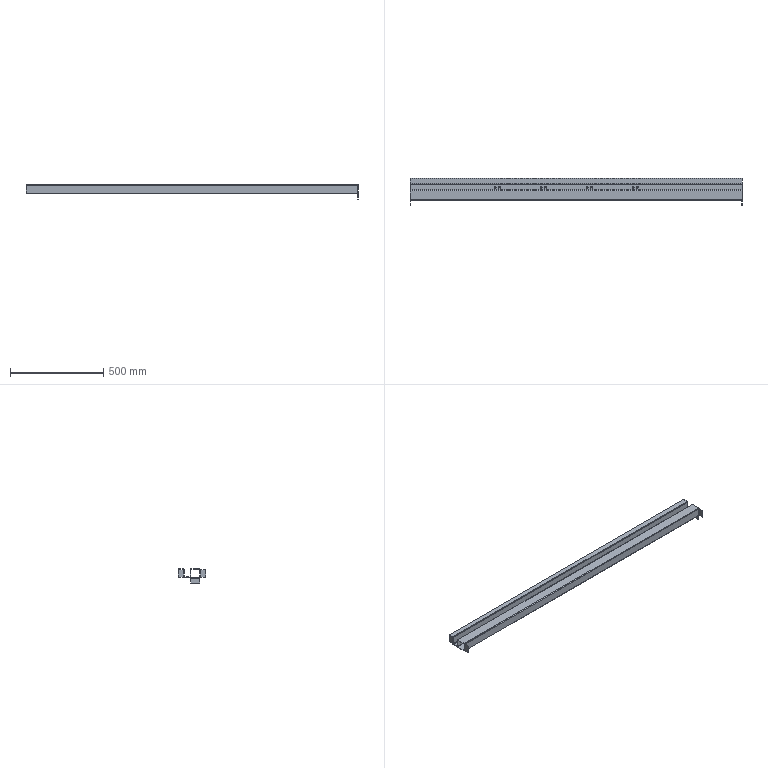Part | SolidWorks | features BaseBody 1 | 1 solid | 197 faces | box 1776 x 144.65 x 75.5 mm | volume 1335995 mm3 | plane 143 | cylinder 54 | commonest cylinder face diameters 6 x16 6.5 x16 2 x11 7 x11